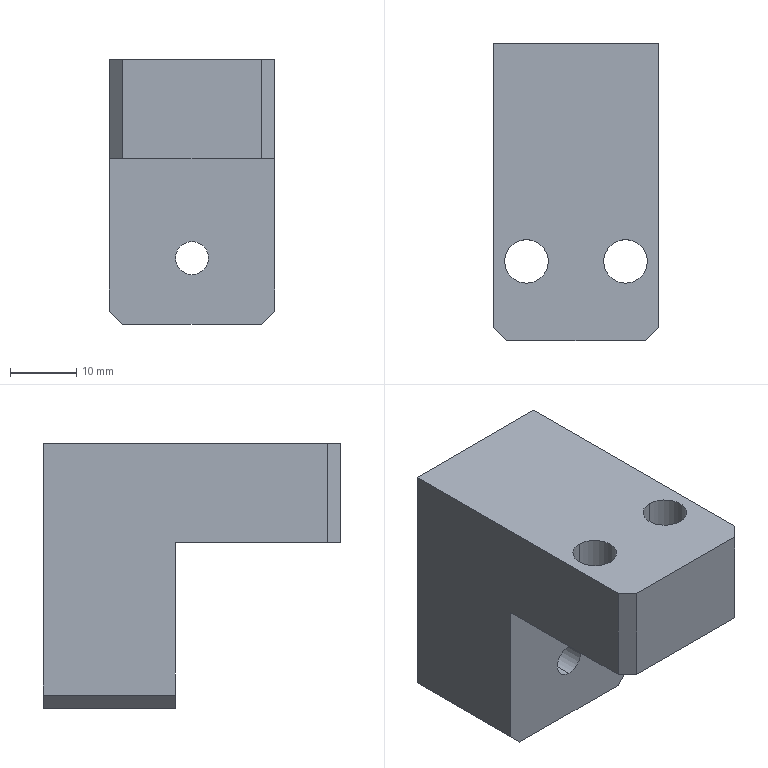Part | SolidWorks | features Chamfer 2, HoleWzd 2, Extrusion 1, ICE 1 | 1 solid | 18 faces | box 25 x 45 x 40 mm | volume 27816 mm3 | plane 12 | cylinder 6 | commonest cylinder face diameters 6.6 x4 5 x2
STEP:
#1=CARTESIAN_POINT('',(20.,-16.3,0.));
#2=VERTEX_POINT('',#1);
#3=CARTESIAN_POINT('',(20.,-9.7,0.));
#4=VERTEX_POINT('',#3);
#5=CARTESIAN_POINT('',(20.,-13.,0.));
#6=DIRECTION('',(0.,0.,-1.));
#7=DIRECTION('',(0.,1.,0.));
#8=AXIS2_PLACEMENT_3D('',#5,#6,#7);
#9=CIRCLE('',#8,3.3);
#10=EDGE_CURVE('',#2,#4,#9,.T.);
#11=ORIENTED_EDGE('',*,*,#10,.F.);
#12=CARTESIAN_POINT('',(20.,-16.3,-15.));
#13=VERTEX_POINT('',#12);
#14=CARTESIAN_POINT('',(20.,-16.3,-15.));
#15=DIRECTION('',(0.,0.,-1.));
#16=VECTOR('',#15,1000.);
#17=LINE('',#14,#16);
#18=EDGE_CURVE('',#2,#13,#17,.T.);
#19=ORIENTED_EDGE('',*,*,#18,.T.);
#20=CARTESIAN_POINT('',(20.,-9.7,-15.));
#21=VERTEX_POINT('',#20);
#22=CARTESIAN_POINT('',(20.,-13.,-15.));
#23=DIRECTION('',(0.,0.,-1.));
#24=DIRECTION('',(0.,1.,0.));
#25=AXIS2_PLACEMENT_3D('',#22,#23,#24);
#26=CIRCLE('',#25,3.3);
#27=EDGE_CURVE('',#13,#21,#26,.T.);
#28=ORIENTED_EDGE('',*,*,#27,.T.);
#29=CARTESIAN_POINT('',(20.,-9.7,-15.));
#30=DIRECTION('',(0.,0.,-1.));
#31=VECTOR('',#30,1000.);
#32=LINE('',#29,#31);
#33=EDGE_CURVE('',#4,#21,#32,.T.);
#34=ORIENTED_EDGE('',*,*,#33,.F.);
#35=EDGE_LOOP('',(#11,#19,#28,#34));
#36=FACE_OUTER_BOUND('',#35,.T.);
#37=CARTESIAN_POINT('',(20.,-13.,-15.));
#38=DIRECTION('',(0.,0.,-1.));
#39=DIRECTION('',(0.,1.,0.));
#40=AXIS2_PLACEMENT_3D('',#37,#38,#39);
#41=CYLINDRICAL_SURFACE('',#40,3.3);
#42=ADVANCED_FACE('',(#36),#41,.F.);
#43=CARTESIAN_POINT('',(5.,-16.3,0.));
#44=VERTEX_POINT('',#43);
#45=CARTESIAN_POINT('',(5.,-9.7,0.));
#46=VERTEX_POINT('',#45);
#47=CARTESIAN_POINT('',(5.,-13.,0.));
#48=DIRECTION('',(0.,0.,-1.));
#49=DIRECTION('',(0.,1.,0.));
#50=AXIS2_PLACEMENT_3D('',#47,#48,#49);
#51=CIRCLE('',#50,3.3);
#52=EDGE_CURVE('',#44,#46,#51,.T.);
#53=ORIENTED_EDGE('',*,*,#52,.F.);
#54=CARTESIAN_POINT('',(5.,-16.3,-15.));
#55=VERTEX_POINT('',#54);
#56=CARTESIAN_POINT('',(5.,-16.3,-15.));
#57=DIRECTION('',(0.,0.,-1.));
#58=VECTOR('',#57,1000.);
#59=LINE('',#56,#58);
#60=EDGE_CURVE('',#44,#55,#59,.T.);
#61=ORIENTED_EDGE('',*,*,#60,.T.);
#62=CARTESIAN_POINT('',(5.,-9.7,-15.));
#63=VERTEX_POINT('',#62);
#64=CARTESIAN_POINT('',(5.,-13.,-15.));
#65=DIRECTION('',(0.,0.,-1.));
#66=DIRECTION('',(0.,1.,0.));
#67=AXIS2_PLACEMENT_3D('',#64,#65,#66);
#68=CIRCLE('',#67,3.3);
#69=EDGE_CURVE('',#55,#63,#68,.T.);
#70=ORIENTED_EDGE('',*,*,#69,.T.);
#71=CARTESIAN_POINT('',(5.,-9.7,-15.));
#72=DIRECTION('',(0.,0.,-1.));
#73=VECTOR('',#72,1000.);
#74=LINE('',#71,#73);
#75=EDGE_CURVE('',#46,#63,#74,.T.);
#76=ORIENTED_EDGE('',*,*,#75,.F.);
#77=EDGE_LOOP('',(#53,#61,#70,#76));
#78=FACE_OUTER_BOUND('',#77,.T.);
#79=CARTESIAN_POINT('',(5.,-13.,-15.));
#80=DIRECTION('',(0.,0.,-1.));
#81=DIRECTION('',(0.,1.,0.));
#82=AXIS2_PLACEMENT_3D('',#79,#80,#81);
#83=CYLINDRICAL_SURFACE('',#82,3.3);
#84=ADVANCED_FACE('',(#78),#83,.F.);
#85=CARTESIAN_POINT('',(12.5,20.,-27.5));
#86=VERTEX_POINT('',#85);
#87=CARTESIAN_POINT('',(12.5,20.,-32.5));
#88=VERTEX_POINT('',#87);
#89=CARTESIAN_POINT('',(12.5,20.,-30.));
#90=DIRECTION('',(0.,-1.,0.));
#91=DIRECTION('',(0.,0.,-1.));
#92=AXIS2_PLACEMENT_3D('',#89,#90,#91);
#93=CIRCLE('',#92,2.5);
#94=EDGE_CURVE('',#86,#88,#93,.T.);
#95=ORIENTED_EDGE('',*,*,#94,.F.);
#96=CARTESIAN_POINT('',(12.5,0.,-27.5));
#97=VERTEX_POINT('',#96);
#98=CARTESIAN_POINT('',(12.5,0.,-27.5));
#99=DIRECTION('',(0.,-1.,0.));
#100=VECTOR('',#99,1000.);
#101=LINE('',#98,#100);
#102=EDGE_CURVE('',#86,#97,#101,.T.);
#103=ORIENTED_EDGE('',*,*,#102,.T.);
#104=CARTESIAN_POINT('',(12.5,0.,-32.5));
#105=VERTEX_POINT('',#104);
#106=CARTESIAN_POINT('',(12.5,0.,-30.));
#107=DIRECTION('',(0.,-1.,0.));
#108=DIRECTION('',(0.,0.,-1.));
#109=AXIS2_PLACEMENT_3D('',#106,#107,#108);
#110=CIRCLE('',#109,2.5);
#111=EDGE_CURVE('',#97,#105,#110,.T.);
#112=ORIENTED_EDGE('',*,*,#111,.T.);
#113=CARTESIAN_POINT('',(12.5,0.,-32.5));
#114=DIRECTION('',(0.,-1.,0.));
#115=VECTOR('',#114,1000.);
#116=LINE('',#113,#115);
#117=EDGE_CURVE('',#88,#105,#116,.T.);
#118=ORIENTED_EDGE('',*,*,#117,.F.);
#119=EDGE_LOOP('',(#95,#103,#112,#118));
#120=FACE_OUTER_BOUND('',#119,.T.);
#121=CARTESIAN_POINT('',(12.5,0.,-30.));
#122=DIRECTION('',(0.,-1.,0.));
#123=DIRECTION('',(0.,0.,-1.));
#124=AXIS2_PLACEMENT_3D('',#121,#122,#123);
#125=CYLINDRICAL_SURFACE('',#124,2.5);
#126=ADVANCED_FACE('',(#120),#125,.F.);
#127=CARTESIAN_POINT('',(0.,0.,-15.));
#128=VERTEX_POINT('',#127);
#129=CARTESIAN_POINT('',(0.,-23.,-15.));
#130=VERTEX_POINT('',#129);
#131=CARTESIAN_POINT('',(0.,0.,-15.));
#132=DIRECTION('',(0.,-1.,0.));
#133=VECTOR('',#132,1000.);
#134=LINE('',#131,#133);
#135=EDGE_CURVE('',#128,#130,#134,.T.);
#136=ORIENTED_EDGE('',*,*,#135,.T.);
#137=CARTESIAN_POINT('',(0.,-23.,0.));
#138=VERTEX_POINT('',#137);
#139=CARTESIAN_POINT('',(0.,-23.,0.));
#140=DIRECTION('',(0.,0.,1.));
#141=VECTOR('',#140,1000.);
#142=LINE('',#139,#141);
#143=EDGE_CURVE('',#130,#138,#142,.T.);
#144=ORIENTED_EDGE('',*,*,#143,.T.);
#145=CARTESIAN_POINT('',(0.,20.,0.));
#146=VERTEX_POINT('',#145);
#147=CARTESIAN_POINT('',(0.,20.,0.));
#148=DIRECTION('',(0.,-1.,0.));
#149=VECTOR('',#148,1000.);
#150=LINE('',#147,#149);
#151=EDGE_CURVE('',#146,#138,#150,.T.);
#152=ORIENTED_EDGE('',*,*,#151,.F.);
#153=CARTESIAN_POINT('',(0.,20.,-38.));
#154=VERTEX_POINT('',#153);
#155=CARTESIAN_POINT('',(0.,20.,0.));
#156=DIRECTION('',(0.,0.,1.));
#157=VECTOR('',#156,1000.);
#158=LINE('',#155,#157);
#159=EDGE_CURVE('',#154,#146,#158,.T.);
#160=ORIENTED_EDGE('',*,*,#159,.F.);
#161=CARTESIAN_POINT('',(0.,0.,-38.));
#162=VERTEX_POINT('',#161);
#163=CARTESIAN_POINT('',(0.,20.,-38.));
#164=DIRECTION('',(0.,-1.,0.));
#165=VECTOR('',#164,1000.);
#166=LINE('',#163,#165);
#167=EDGE_CURVE('',#154,#162,#166,.T.);
#168=ORIENTED_EDGE('',*,*,#167,.T.);
#169=CARTESIAN_POINT('',(0.,0.,0.));
#170=DIRECTION('',(0.,0.,1.));
#171=VECTOR('',#170,1000.);
#172=LINE('',#169,#171);
#173=EDGE_CURVE('',#162,#128,#172,.T.);
#174=ORIENTED_EDGE('',*,*,#173,.T.);
#175=EDGE_LOOP('',(#136,#144,#152,#160,#168,#174));
#176=FACE_OUTER_BOUND('',#175,.T.);
#177=CARTESIAN_POINT('',(0.,20.,0.));
#178=DIRECTION('',(1.,0.,0.));
#179=DIRECTION('',(0.,0.,-1.));
#180=AXIS2_PLACEMENT_3D('',#177,#178,#179);
#181=PLANE('',#180);
#182=ADVANCED_FACE('',(#176),#181,.F.);
#183=CARTESIAN_POINT('',(20.,-13.,0.));
#184=DIRECTION('',(0.,0.,-1.));
#185=DIRECTION('',(0.,1.,0.));
#186=AXIS2_PLACEMENT_3D('',#183,#184,#185);
#187=CIRCLE('',#186,3.3);
#188=EDGE_CURVE('',#4,#2,#187,.T.);
#189=ORIENTED_EDGE('',*,*,#188,.T.);
#190=ORIENTED_EDGE('',*,*,#10,.T.);
#191=EDGE_LOOP('',(#189,#190));
#192=FACE_BOUND('',#191,.T.);
#193=CARTESIAN_POINT('',(5.,-13.,0.));
#194=DIRECTION('',(0.,0.,-1.));
#195=DIRECTION('',(0.,1.,0.));
#196=AXIS2_PLACEMENT_3D('',#193,#194,#195);
#197=CIRCLE('',#196,3.3);
#198=EDGE_CURVE('',#46,#44,#197,.T.);
#199=ORIENTED_EDGE('',*,*,#198,.T.);
#200=ORIENTED_EDGE('',*,*,#52,.T.);
#201=EDGE_LOOP('',(#199,#200));
#202=FACE_BOUND('',#201,.T.);
#203=ORIENTED_EDGE('',*,*,#151,.T.);
#204=CARTESIAN_POINT('',(2.,-25.,0.));
#205=VERTEX_POINT('',#204);
#206=CARTESIAN_POINT('',(0.,-23.,0.));
#207=DIRECTION('',(0.7071,-0.7071,0.));
#208=VECTOR('',#207,1000.);
#209=LINE('',#206,#208);
#210=EDGE_CURVE('',#138,#205,#209,.T.);
#211=ORIENTED_EDGE('',*,*,#210,.T.);
#212=CARTESIAN_POINT('',(23.,-25.,0.));
#213=VERTEX_POINT('',#212);
#214=CARTESIAN_POINT('',(-29.155,-25.,0.));
#215=DIRECTION('',(1.,0.,0.));
#216=VECTOR('',#215,1000.);
#217=LINE('',#214,#216);
#218=EDGE_CURVE('',#205,#213,#217,.T.);
#219=ORIENTED_EDGE('',*,*,#218,.T.);
#220=CARTESIAN_POINT('',(25.,-23.,0.));
#221=VERTEX_POINT('',#220);
#222=CARTESIAN_POINT('',(25.,-23.,0.));
#223=DIRECTION('',(0.7071,0.7071,0.));
#224=VECTOR('',#223,1000.);
#225=LINE('',#222,#224);
#226=EDGE_CURVE('',#213,#221,#225,.T.);
#227=ORIENTED_EDGE('',*,*,#226,.T.);
#228=CARTESIAN_POINT('',(25.,20.,0.));
#229=VERTEX_POINT('',#228);
#230=CARTESIAN_POINT('',(25.,20.,0.));
#231=DIRECTION('',(0.,-1.,0.));
#232=VECTOR('',#231,1000.);
#233=LINE('',#230,#232);
#234=EDGE_CURVE('',#229,#221,#233,.T.);
#235=ORIENTED_EDGE('',*,*,#234,.F.);
#236=CARTESIAN_POINT('',(0.,20.,0.));
#237=DIRECTION('',(1.,0.,0.));
#238=VECTOR('',#237,1000.);
#239=LINE('',#236,#238);
#240=EDGE_CURVE('',#146,#229,#239,.T.);
#241=ORIENTED_EDGE('',*,*,#240,.F.);
#242=EDGE_LOOP('',(#203,#211,#219,#227,#235,#241));
#243=FACE_OUTER_BOUND('',#242,.T.);
#244=CARTESIAN_POINT('',(0.,20.,0.));
#245=DIRECTION('',(0.,0.,-1.));
#246=DIRECTION('',(-1.,0.,0.));
#247=AXIS2_PLACEMENT_3D('',#244,#245,#246);
#248=PLANE('',#247);
#249=ADVANCED_FACE('',(#192,#202,#243),#248,.F.);
#250=ORIENTED_EDGE('',*,*,#234,.T.);
#251=CARTESIAN_POINT('',(25.,-23.,-15.));
#252=VERTEX_POINT('',#251);
#253=CARTESIAN_POINT('',(25.,-23.,-15.));
#254=DIRECTION('',(0.,0.,-1.));
#255=VECTOR('',#254,1000.);
#256=LINE('',#253,#255);
#257=EDGE_CURVE('',#221,#252,#256,.T.);
#258=ORIENTED_EDGE('',*,*,#257,.T.);
#259=CARTESIAN_POINT('',(25.,0.,-15.));
#260=VERTEX_POINT('',#259);
#261=CARTESIAN_POINT('',(25.,0.,-15.));
#262=DIRECTION('',(0.,1.,0.));
#263=VECTOR('',#262,1000.);
#264=LINE('',#261,#263);
#265=EDGE_CURVE('',#252,#260,#264,.T.);
#266=ORIENTED_EDGE('',*,*,#265,.T.);
#267=CARTESIAN_POINT('',(25.,0.,-38.));
#268=VERTEX_POINT('',#267);
#269=CARTESIAN_POINT('',(25.,0.,0.));
#270=DIRECTION('',(0.,0.,-1.));
#271=VECTOR('',#270,1000.);
#272=LINE('',#269,#271);
#273=EDGE_CURVE('',#260,#268,#272,.T.);
#274=ORIENTED_EDGE('',*,*,#273,.T.);
#275=CARTESIAN_POINT('',(25.,20.,-38.));
#276=VERTEX_POINT('',#275);
#277=CARTESIAN_POINT('',(25.,20.,-38.));
#278=DIRECTION('',(0.,1.,0.));
#279=VECTOR('',#278,1000.);
#280=LINE('',#277,#279);
#281=EDGE_CURVE('',#268,#276,#280,.T.);
#282=ORIENTED_EDGE('',*,*,#281,.T.);
#283=CARTESIAN_POINT('',(25.,20.,0.));
#284=DIRECTION('',(0.,0.,-1.));
#285=VECTOR('',#284,1000.);
#286=LINE('',#283,#285);
#287=EDGE_CURVE('',#229,#276,#286,.T.);
#288=ORIENTED_EDGE('',*,*,#287,.F.);
#289=EDGE_LOOP('',(#250,#258,#266,#274,#282,#288));
#290=FACE_OUTER_BOUND('',#289,.T.);
#291=CARTESIAN_POINT('',(25.,20.,0.));
#292=DIRECTION('',(-1.,0.,0.));
#293=DIRECTION('',(0.,0.,1.));
#294=AXIS2_PLACEMENT_3D('',#291,#292,#293);
#295=PLANE('',#294);
#296=ADVANCED_FACE('',(#290),#295,.F.);
#297=CARTESIAN_POINT('',(23.,0.,-40.));
#298=VERTEX_POINT('',#297);
#299=CARTESIAN_POINT('',(2.,0.,-40.));
#300=VERTEX_POINT('',#299);
#301=CARTESIAN_POINT('',(0.,0.,-40.));
#302=DIRECTION('',(-1.,0.,0.));
#303=VECTOR('',#302,1000.);
#304=LINE('',#301,#303);
#305=EDGE_CURVE('',#298,#300,#304,.T.);
#306=ORIENTED_EDGE('',*,*,#305,.T.);
#307=CARTESIAN_POINT('',(2.,20.,-40.));
#308=VERTEX_POINT('',#307);
#309=CARTESIAN_POINT('',(2.,20.,-40.));
#310=DIRECTION('',(0.,1.,0.));
#311=VECTOR('',#310,1000.);
#312=LINE('',#309,#311);
#313=EDGE_CURVE('',#300,#308,#312,.T.);
#314=ORIENTED_EDGE('',*,*,#313,.T.);
#315=CARTESIAN_POINT('',(23.,20.,-40.));
#316=VERTEX_POINT('',#315);
#317=CARTESIAN_POINT('',(0.,20.,-40.));
#318=DIRECTION('',(-1.,0.,0.));
#319=VECTOR('',#318,1000.);
#320=LINE('',#317,#319);
#321=EDGE_CURVE('',#316,#308,#320,.T.);
#322=ORIENTED_EDGE('',*,*,#321,.F.);
#323=CARTESIAN_POINT('',(23.,20.,-40.));
#324=DIRECTION('',(0.,-1.,0.));
#325=VECTOR('',#324,1000.);
#326=LINE('',#323,#325);
#327=EDGE_CURVE('',#316,#298,#326,.T.);
#328=ORIENTED_EDGE('',*,*,#327,.T.);
#329=EDGE_LOOP('',(#306,#314,#322,#328));
#330=FACE_OUTER_BOUND('',#329,.T.);
#331=CARTESIAN_POINT('',(0.,20.,-40.));
#332=DIRECTION('',(0.,0.,1.));
#333=DIRECTION('',(1.,0.,0.));
#334=AXIS2_PLACEMENT_3D('',#331,#332,#333);
#335=PLANE('',#334);
#336=ADVANCED_FACE('',(#330),#335,.F.);
#337=CARTESIAN_POINT('',(12.5,20.,-30.));
#338=DIRECTION('',(0.,-1.,0.));
#339=DIRECTION('',(0.,0.,-1.));
#340=AXIS2_PLACEMENT_3D('',#337,#338,#339);
#341=CIRCLE('',#340,2.5);
#342=EDGE_CURVE('',#88,#86,#341,.T.);
#343=ORIENTED_EDGE('',*,*,#342,.T.);
#344=ORIENTED_EDGE('',*,*,#94,.T.);
#345=EDGE_LOOP('',(#343,#344));
#346=FACE_BOUND('',#345,.T.);
#347=ORIENTED_EDGE('',*,*,#321,.T.);
#348=CARTESIAN_POINT('',(0.,20.,-38.));
#349=DIRECTION('',(-0.7071,0.,0.7071));
#350=VECTOR('',#349,1000.);
#351=LINE('',#348,#350);
#352=EDGE_CURVE('',#308,#154,#351,.T.);
#353=ORIENTED_EDGE('',*,*,#352,.T.);
#354=ORIENTED_EDGE('',*,*,#159,.T.);
#355=ORIENTED_EDGE('',*,*,#240,.T.);
#356=ORIENTED_EDGE('',*,*,#287,.T.);
#357=CARTESIAN_POINT('',(23.,20.,-40.));
#358=DIRECTION('',(-0.7071,0.,-0.7071));
#359=VECTOR('',#358,1000.);
#360=LINE('',#357,#359);
#361=EDGE_CURVE('',#276,#316,#360,.T.);
#362=ORIENTED_EDGE('',*,*,#361,.T.);
#363=EDGE_LOOP('',(#347,#353,#354,#355,#356,#362));
#364=FACE_OUTER_BOUND('',#363,.T.);
#365=CARTESIAN_POINT('',(0.,20.,0.));
#366=DIRECTION('',(0.,-1.,0.));
#367=DIRECTION('',(0.,0.,-1.));
#368=AXIS2_PLACEMENT_3D('',#365,#366,#367);
#369=PLANE('',#368);
#370=ADVANCED_FACE('',(#346,#364),#369,.F.);
#371=CARTESIAN_POINT('',(-29.155,0.,-15.));
#372=DIRECTION('',(1.,0.,0.));
#373=VECTOR('',#372,1000.);
#374=LINE('',#371,#373);
#375=EDGE_CURVE('',#128,#260,#374,.T.);
#376=ORIENTED_EDGE('',*,*,#375,.F.);
#377=ORIENTED_EDGE('',*,*,#173,.F.);
#378=CARTESIAN_POINT('',(-19.,0.,-19.));
#379=DIRECTION('',(0.7071,0.,-0.7071));
#380=VECTOR('',#379,1000.);
#381=LINE('',#378,#380);
#382=EDGE_CURVE('',#162,#300,#381,.T.);
#383=ORIENTED_EDGE('',*,*,#382,.T.);
#384=ORIENTED_EDGE('',*,*,#305,.F.);
#385=CARTESIAN_POINT('',(31.5,0.,-31.5));
#386=DIRECTION('',(0.7071,0.,0.7071));
#387=VECTOR('',#386,1000.);
#388=LINE('',#385,#387);
#389=EDGE_CURVE('',#298,#268,#388,.T.);
#390=ORIENTED_EDGE('',*,*,#389,.T.);
#391=ORIENTED_EDGE('',*,*,#273,.F.);
#392=EDGE_LOOP('',(#376,#377,#383,#384,#390,#391));
#393=FACE_OUTER_BOUND('',#392,.T.);
#394=CARTESIAN_POINT('',(12.5,0.,-30.));
#395=DIRECTION('',(0.,-1.,0.));
#396=DIRECTION('',(0.,0.,-1.));
#397=AXIS2_PLACEMENT_3D('',#394,#395,#396);
#398=CIRCLE('',#397,2.5);
#399=EDGE_CURVE('',#105,#97,#398,.T.);
#400=ORIENTED_EDGE('',*,*,#399,.F.);
#401=ORIENTED_EDGE('',*,*,#111,.F.);
#402=EDGE_LOOP('',(#400,#401));
#403=FACE_BOUND('',#402,.T.);
#404=CARTESIAN_POINT('',(0.,0.,0.));
#405=DIRECTION('',(0.,-1.,0.));
#406=DIRECTION('',(0.,0.,-1.));
#407=AXIS2_PLACEMENT_3D('',#404,#405,#406);
#408=PLANE('',#407);
#409=ADVANCED_FACE('',(#393,#403),#408,.T.);
#410=ORIENTED_EDGE('',*,*,#352,.F.);
#411=ORIENTED_EDGE('',*,*,#313,.F.);
#412=ORIENTED_EDGE('',*,*,#382,.F.);
#413=ORIENTED_EDGE('',*,*,#167,.F.);
#414=EDGE_LOOP('',(#410,#411,#412,#413));
#415=FACE_OUTER_BOUND('',#414,.T.);
#416=CARTESIAN_POINT('',(0.,20.,-38.));
#417=DIRECTION('',(0.7071,0.,0.7071));
#418=DIRECTION('',(0.,-1.,0.));
#419=AXIS2_PLACEMENT_3D('',#416,#417,#418);
#420=PLANE('',#419);
#421=ADVANCED_FACE('',(#415),#420,.F.);
#422=ORIENTED_EDGE('',*,*,#361,.F.);
#423=ORIENTED_EDGE('',*,*,#281,.F.);
#424=ORIENTED_EDGE('',*,*,#389,.F.);
#425=ORIENTED_EDGE('',*,*,#327,.F.);
#426=EDGE_LOOP('',(#422,#423,#424,#425));
#427=FACE_OUTER_BOUND('',#426,.T.);
#428=CARTESIAN_POINT('',(23.,20.,-40.));
#429=DIRECTION('',(-0.7071,0.,0.7071));
#430=DIRECTION('',(0.,-1.,0.));
#431=AXIS2_PLACEMENT_3D('',#428,#429,#430);
#432=PLANE('',#431);
#433=ADVANCED_FACE('',(#427),#432,.F.);
#434=ORIENTED_EDGE('',*,*,#102,.F.);
#435=ORIENTED_EDGE('',*,*,#342,.F.);
#436=ORIENTED_EDGE('',*,*,#117,.T.);
#437=ORIENTED_EDGE('',*,*,#399,.T.);
#438=EDGE_LOOP('',(#434,#435,#436,#437));
#439=FACE_OUTER_BOUND('',#438,.T.);
#440=CARTESIAN_POINT('',(12.5,0.,-30.));
#441=DIRECTION('',(0.,-1.,0.));
#442=DIRECTION('',(0.,0.,-1.));
#443=AXIS2_PLACEMENT_3D('',#440,#441,#442);
#444=CYLINDRICAL_SURFACE('',#443,2.5);
#445=ADVANCED_FACE('',(#439),#444,.F.);
#446=CARTESIAN_POINT('',(20.,-13.,-15.));
#447=DIRECTION('',(0.,0.,-1.));
#448=DIRECTION('',(0.,1.,0.));
#449=AXIS2_PLACEMENT_3D('',#446,#447,#448);
#450=CIRCLE('',#449,3.3);
#451=EDGE_CURVE('',#21,#13,#450,.T.);
#452=ORIENTED_EDGE('',*,*,#451,.F.);
#453=ORIENTED_EDGE('',*,*,#27,.F.);
#454=EDGE_LOOP('',(#452,#453));
#455=FACE_BOUND('',#454,.T.);
#456=CARTESIAN_POINT('',(5.,-13.,-15.));
#457=DIRECTION('',(0.,0.,-1.));
#458=DIRECTION('',(0.,1.,0.));
#459=AXIS2_PLACEMENT_3D('',#456,#457,#458);
#460=CIRCLE('',#459,3.3);
#461=EDGE_CURVE('',#63,#55,#460,.T.);
#462=ORIENTED_EDGE('',*,*,#461,.F.);
#463=ORIENTED_EDGE('',*,*,#69,.F.);
#464=EDGE_LOOP('',(#462,#463));
#465=FACE_BOUND('',#464,.T.);
#466=CARTESIAN_POINT('',(2.,-25.,-15.));
#467=VERTEX_POINT('',#466);
#468=CARTESIAN_POINT('',(23.,-25.,-15.));
#469=VERTEX_POINT('',#468);
#470=CARTESIAN_POINT('',(-29.155,-25.,-15.));
#471=DIRECTION('',(1.,0.,0.));
#472=VECTOR('',#471,1000.);
#473=LINE('',#470,#472);
#474=EDGE_CURVE('',#467,#469,#473,.T.);
#475=ORIENTED_EDGE('',*,*,#474,.F.);
#476=CARTESIAN_POINT('',(-26.077,3.077,-15.));
#477=DIRECTION('',(-0.7071,0.7071,0.));
#478=VECTOR('',#477,1000.);
#479=LINE('',#476,#478);
#480=EDGE_CURVE('',#467,#130,#479,.T.);
#481=ORIENTED_EDGE('',*,*,#480,.T.);
#482=ORIENTED_EDGE('',*,*,#135,.F.);
#483=ORIENTED_EDGE('',*,*,#375,.T.);
#484=ORIENTED_EDGE('',*,*,#265,.F.);
#485=CARTESIAN_POINT('',(9.423,-38.577,-15.));
#486=DIRECTION('',(-0.7071,-0.7071,0.));
#487=VECTOR('',#486,1000.);
#488=LINE('',#485,#487);
#489=EDGE_CURVE('',#252,#469,#488,.T.);
#490=ORIENTED_EDGE('',*,*,#489,.T.);
#491=EDGE_LOOP('',(#475,#481,#482,#483,#484,#490));
#492=FACE_OUTER_BOUND('',#491,.T.);
#493=CARTESIAN_POINT('',(-29.155,0.,-15.));
#494=DIRECTION('',(0.,0.,-1.));
#495=DIRECTION('',(0.,1.,0.));
#496=AXIS2_PLACEMENT_3D('',#493,#494,#495);
#497=PLANE('',#496);
#498=ADVANCED_FACE('',(#455,#465,#492),#497,.T.);
#499=ORIENTED_EDGE('',*,*,#218,.F.);
#500=CARTESIAN_POINT('',(2.,-25.,-15.));
#501=DIRECTION('',(0.,0.,-1.));
#502=VECTOR('',#501,1000.);
#503=LINE('',#500,#502);
#504=EDGE_CURVE('',#205,#467,#503,.T.);
#505=ORIENTED_EDGE('',*,*,#504,.T.);
#506=ORIENTED_EDGE('',*,*,#474,.T.);
#507=CARTESIAN_POINT('',(23.,-25.,0.));
#508=DIRECTION('',(0.,0.,1.));
#509=VECTOR('',#508,1000.);
#510=LINE('',#507,#509);
#511=EDGE_CURVE('',#469,#213,#510,.T.);
#512=ORIENTED_EDGE('',*,*,#511,.T.);
#513=EDGE_LOOP('',(#499,#505,#506,#512));
#514=FACE_OUTER_BOUND('',#513,.T.);
#515=CARTESIAN_POINT('',(-29.155,-25.,0.));
#516=DIRECTION('',(0.,-1.,0.));
#517=DIRECTION('',(0.,0.,-1.));
#518=AXIS2_PLACEMENT_3D('',#515,#516,#517);
#519=PLANE('',#518);
#520=ADVANCED_FACE('',(#514),#519,.T.);
#521=ORIENTED_EDGE('',*,*,#60,.F.);
#522=ORIENTED_EDGE('',*,*,#198,.F.);
#523=ORIENTED_EDGE('',*,*,#75,.T.);
#524=ORIENTED_EDGE('',*,*,#461,.T.);
#525=EDGE_LOOP('',(#521,#522,#523,#524));
#526=FACE_OUTER_BOUND('',#525,.T.);
#527=CARTESIAN_POINT('',(5.,-13.,-15.));
#528=DIRECTION('',(0.,0.,-1.));
#529=DIRECTION('',(0.,1.,0.));
#530=AXIS2_PLACEMENT_3D('',#527,#528,#529);
#531=CYLINDRICAL_SURFACE('',#530,3.3);
#532=ADVANCED_FACE('',(#526),#531,.F.);
#533=ORIENTED_EDGE('',*,*,#18,.F.);
#534=ORIENTED_EDGE('',*,*,#188,.F.);
#535=ORIENTED_EDGE('',*,*,#33,.T.);
#536=ORIENTED_EDGE('',*,*,#451,.T.);
#537=EDGE_LOOP('',(#533,#534,#535,#536));
#538=FACE_OUTER_BOUND('',#537,.T.);
#539=CARTESIAN_POINT('',(20.,-13.,-15.));
#540=DIRECTION('',(0.,0.,-1.));
#541=DIRECTION('',(0.,1.,0.));
#542=AXIS2_PLACEMENT_3D('',#539,#540,#541);
#543=CYLINDRICAL_SURFACE('',#542,3.3);
#544=ADVANCED_FACE('',(#538),#543,.F.);
#545=ORIENTED_EDGE('',*,*,#480,.F.);
#546=ORIENTED_EDGE('',*,*,#504,.F.);
#547=ORIENTED_EDGE('',*,*,#210,.F.);
#548=ORIENTED_EDGE('',*,*,#143,.F.);
#549=EDGE_LOOP('',(#545,#546,#547,#548));
#550=FACE_OUTER_BOUND('',#549,.T.);
#551=CARTESIAN_POINT('',(0.,-23.,0.));
#552=DIRECTION('',(-0.7071,-0.7071,0.));
#553=DIRECTION('',(0.,0.,-1.));
#554=AXIS2_PLACEMENT_3D('',#551,#552,#553);
#555=PLANE('',#554);
#556=ADVANCED_FACE('',(#550),#555,.T.);
#557=ORIENTED_EDGE('',*,*,#226,.F.);
#558=ORIENTED_EDGE('',*,*,#511,.F.);
#559=ORIENTED_EDGE('',*,*,#489,.F.);
#560=ORIENTED_EDGE('',*,*,#257,.F.);
#561=EDGE_LOOP('',(#557,#558,#559,#560));
#562=FACE_OUTER_BOUND('',#561,.T.);
#563=CARTESIAN_POINT('',(25.,-23.,0.));
#564=DIRECTION('',(0.7071,-0.7071,0.));
#565=DIRECTION('',(0.,0.,1.));
#566=AXIS2_PLACEMENT_3D('',#563,#564,#565);
#567=PLANE('',#566);
#568=ADVANCED_FACE('',(#562),#567,.T.);
#569=CLOSED_SHELL('',(#42,#84,#126,#182,#249,#296,#336,#370,#409,#421,#433,#445,#498,#520,#532,#544,#556,#568));
#570=MANIFOLD_SOLID_BREP('',#569);
#571=CARTESIAN_POINT('',(0.,0.,0.));
#572=DIRECTION('',(0.,0.,1.));
#573=DIRECTION('',(1.,0.,0.));
#574=AXIS2_PLACEMENT_3D('',#571,#572,#573);
#575=(LENGTH_UNIT()NAMED_UNIT(*)SI_UNIT(.MILLI.,.METRE.));
#576=UNCERTAINTY_MEASURE_WITH_UNIT(LENGTH_MEASURE(0.00001),#575,'','');
#577=(NAMED_UNIT(*)PLANE_ANGLE_UNIT()SI_UNIT($,.RADIAN.));
#578=(NAMED_UNIT(*)SI_UNIT($,.STERADIAN.)SOLID_ANGLE_UNIT());
#579=(GEOMETRIC_REPRESENTATION_CONTEXT(3)GLOBAL_UNCERTAINTY_ASSIGNED_CONTEXT((#576))GLOBAL_UNIT_ASSIGNED_CONTEXT((#575,#577,#578))REPRESENTATION_CONTEXT('',''));
#580=ADVANCED_BREP_SHAPE_REPRESENTATION('',(#570,#574),#579);